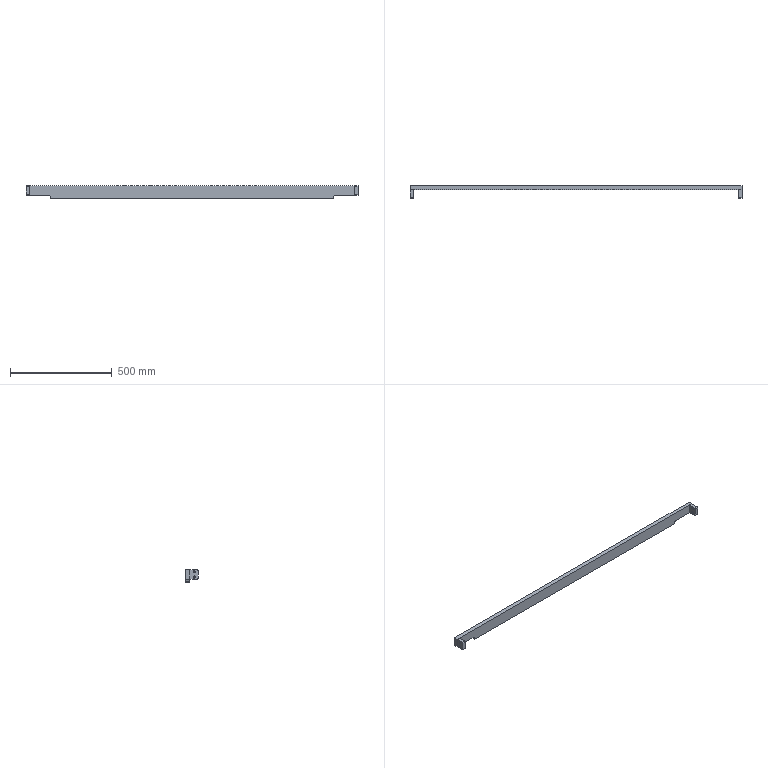Part | SolidWorks | features BaseBody 3 | 3 solids | 36 faces | box 1632 x 60 x 60 mm | volume 1939285 mm3 | plane 22 | cylinder 14 | commonest cylinder face diameters 10.2 x8 10 x4 20 x2
STEP:
#1=CARTESIAN_POINT('',(816.,-10.,30.));
#2=VERTEX_POINT('',#1);
#3=CARTESIAN_POINT('',(816.,-10.,-15.));
#4=VERTEX_POINT('',#3);
#5=CARTESIAN_POINT('',(816.,-10.,-30.));
#6=DIRECTION('',(0.,0.,-1.));
#7=VECTOR('',#6,1000.);
#8=LINE('',#5,#7);
#9=EDGE_CURVE('',#2,#4,#8,.T.);
#10=ORIENTED_EDGE('',*,*,#9,.T.);
#11=CARTESIAN_POINT('',(816.,10.,-15.));
#12=VERTEX_POINT('',#11);
#13=CARTESIAN_POINT('',(816.,-10.,-15.));
#14=DIRECTION('',(0.,1.,0.));
#15=VECTOR('',#14,1000.);
#16=LINE('',#13,#15);
#17=EDGE_CURVE('',#4,#12,#16,.T.);
#18=ORIENTED_EDGE('',*,*,#17,.T.);
#19=CARTESIAN_POINT('',(816.,10.,30.));
#20=VERTEX_POINT('',#19);
#21=CARTESIAN_POINT('',(816.,10.,-30.));
#22=DIRECTION('',(0.,0.,-1.));
#23=VECTOR('',#22,1000.);
#24=LINE('',#21,#23);
#25=EDGE_CURVE('',#20,#12,#24,.T.);
#26=ORIENTED_EDGE('',*,*,#25,.F.);
#27=CARTESIAN_POINT('',(816.,10.,30.));
#28=DIRECTION('',(0.,-1.,0.));
#29=VECTOR('',#28,1000.);
#30=LINE('',#27,#29);
#31=EDGE_CURVE('',#20,#2,#30,.T.);
#32=ORIENTED_EDGE('',*,*,#31,.T.);
#33=EDGE_LOOP('',(#10,#18,#26,#32));
#34=FACE_OUTER_BOUND('',#33,.T.);
#35=CARTESIAN_POINT('',(816.,10.,-30.));
#36=DIRECTION('',(-1.,0.,0.));
#37=DIRECTION('',(0.,0.,1.));
#38=AXIS2_PLACEMENT_3D('',#35,#36,#37);
#39=PLANE('',#38);
#40=ADVANCED_FACE('',(#34),#39,.F.);
#41=CARTESIAN_POINT('',(696.,-10.,-30.));
#42=VERTEX_POINT('',#41);
#43=CARTESIAN_POINT('',(-696.,-10.,-30.));
#44=VERTEX_POINT('',#43);
#45=CARTESIAN_POINT('',(-816.,-10.,-30.));
#46=DIRECTION('',(-1.,0.,0.));
#47=VECTOR('',#46,1000.);
#48=LINE('',#45,#47);
#49=EDGE_CURVE('',#42,#44,#48,.T.);
#50=ORIENTED_EDGE('',*,*,#49,.T.);
#51=CARTESIAN_POINT('',(-696.,10.,-30.));
#52=VERTEX_POINT('',#51);
#53=CARTESIAN_POINT('',(-696.,-10.,-30.));
#54=DIRECTION('',(0.,1.,0.));
#55=VECTOR('',#54,1000.);
#56=LINE('',#53,#55);
#57=EDGE_CURVE('',#44,#52,#56,.T.);
#58=ORIENTED_EDGE('',*,*,#57,.T.);
#59=CARTESIAN_POINT('',(696.,10.,-30.));
#60=VERTEX_POINT('',#59);
#61=CARTESIAN_POINT('',(-816.,10.,-30.));
#62=DIRECTION('',(-1.,0.,0.));
#63=VECTOR('',#62,1000.);
#64=LINE('',#61,#63);
#65=EDGE_CURVE('',#60,#52,#64,.T.);
#66=ORIENTED_EDGE('',*,*,#65,.F.);
#67=CARTESIAN_POINT('',(696.,-10.,-30.));
#68=DIRECTION('',(0.,1.,0.));
#69=VECTOR('',#68,1000.);
#70=LINE('',#67,#69);
#71=EDGE_CURVE('',#42,#60,#70,.T.);
#72=ORIENTED_EDGE('',*,*,#71,.F.);
#73=EDGE_LOOP('',(#50,#58,#66,#72));
#74=FACE_OUTER_BOUND('',#73,.T.);
#75=CARTESIAN_POINT('',(-816.,10.,-30.));
#76=DIRECTION('',(0.,0.,1.));
#77=DIRECTION('',(1.,0.,0.));
#78=AXIS2_PLACEMENT_3D('',#75,#76,#77);
#79=PLANE('',#78);
#80=ADVANCED_FACE('',(#74),#79,.F.);
#81=CARTESIAN_POINT('',(-816.,10.,-15.));
#82=VERTEX_POINT('',#81);
#83=CARTESIAN_POINT('',(-816.,10.,30.));
#84=VERTEX_POINT('',#83);
#85=CARTESIAN_POINT('',(-816.,10.,-30.));
#86=DIRECTION('',(0.,0.,1.));
#87=VECTOR('',#86,1000.);
#88=LINE('',#85,#87);
#89=EDGE_CURVE('',#82,#84,#88,.T.);
#90=ORIENTED_EDGE('',*,*,#89,.F.);
#91=CARTESIAN_POINT('',(-816.,-10.,-15.));
#92=VERTEX_POINT('',#91);
#93=CARTESIAN_POINT('',(-816.,-10.,-15.));
#94=DIRECTION('',(0.,1.,0.));
#95=VECTOR('',#94,1000.);
#96=LINE('',#93,#95);
#97=EDGE_CURVE('',#92,#82,#96,.T.);
#98=ORIENTED_EDGE('',*,*,#97,.F.);
#99=CARTESIAN_POINT('',(-816.,-10.,30.));
#100=VERTEX_POINT('',#99);
#101=CARTESIAN_POINT('',(-816.,-10.,-30.));
#102=DIRECTION('',(0.,0.,1.));
#103=VECTOR('',#102,1000.);
#104=LINE('',#101,#103);
#105=EDGE_CURVE('',#92,#100,#104,.T.);
#106=ORIENTED_EDGE('',*,*,#105,.T.);
#107=CARTESIAN_POINT('',(-816.,10.,30.));
#108=DIRECTION('',(0.,-1.,0.));
#109=VECTOR('',#108,1000.);
#110=LINE('',#107,#109);
#111=EDGE_CURVE('',#84,#100,#110,.T.);
#112=ORIENTED_EDGE('',*,*,#111,.F.);
#113=EDGE_LOOP('',(#90,#98,#106,#112));
#114=FACE_OUTER_BOUND('',#113,.T.);
#115=CARTESIAN_POINT('',(-816.,10.,-30.));
#116=DIRECTION('',(1.,0.,0.));
#117=DIRECTION('',(0.,0.,-1.));
#118=AXIS2_PLACEMENT_3D('',#115,#116,#117);
#119=PLANE('',#118);
#120=ADVANCED_FACE('',(#114),#119,.F.);
#121=CARTESIAN_POINT('',(-816.,-10.,30.));
#122=DIRECTION('',(1.,0.,0.));
#123=VECTOR('',#122,1000.);
#124=LINE('',#121,#123);
#125=EDGE_CURVE('',#100,#2,#124,.T.);
#126=ORIENTED_EDGE('',*,*,#125,.T.);
#127=ORIENTED_EDGE('',*,*,#31,.F.);
#128=CARTESIAN_POINT('',(-816.,10.,30.));
#129=DIRECTION('',(1.,0.,0.));
#130=VECTOR('',#129,1000.);
#131=LINE('',#128,#130);
#132=EDGE_CURVE('',#84,#20,#131,.T.);
#133=ORIENTED_EDGE('',*,*,#132,.F.);
#134=ORIENTED_EDGE('',*,*,#111,.T.);
#135=EDGE_LOOP('',(#126,#127,#133,#134));
#136=FACE_OUTER_BOUND('',#135,.T.);
#137=CARTESIAN_POINT('',(-816.,10.,30.));
#138=DIRECTION('',(0.,0.,-1.));
#139=DIRECTION('',(-1.,0.,0.));
#140=AXIS2_PLACEMENT_3D('',#137,#138,#139);
#141=PLANE('',#140);
#142=ADVANCED_FACE('',(#136),#141,.F.);
#143=CARTESIAN_POINT('',(-696.,10.,-25.));
#144=VERTEX_POINT('',#143);
#145=CARTESIAN_POINT('',(-696.,10.,-30.));
#146=DIRECTION('',(0.,0.,-1.));
#147=VECTOR('',#146,1000.);
#148=LINE('',#145,#147);
#149=EDGE_CURVE('',#144,#52,#148,.T.);
#150=ORIENTED_EDGE('',*,*,#149,.F.);
#151=CARTESIAN_POINT('',(-706.,10.,-15.));
#152=VERTEX_POINT('',#151);
#153=CARTESIAN_POINT('',(-706.,10.,-25.));
#154=DIRECTION('',(0.,1.,0.));
#155=DIRECTION('',(0.,0.,1.));
#156=AXIS2_PLACEMENT_3D('',#153,#154,#155);
#157=CIRCLE('',#156,10.);
#158=EDGE_CURVE('',#152,#144,#157,.T.);
#159=ORIENTED_EDGE('',*,*,#158,.F.);
#160=CARTESIAN_POINT('',(-816.,10.,-15.));
#161=DIRECTION('',(1.,0.,0.));
#162=VECTOR('',#161,1000.);
#163=LINE('',#160,#162);
#164=EDGE_CURVE('',#82,#152,#163,.T.);
#165=ORIENTED_EDGE('',*,*,#164,.F.);
#166=ORIENTED_EDGE('',*,*,#89,.T.);
#167=ORIENTED_EDGE('',*,*,#132,.T.);
#168=ORIENTED_EDGE('',*,*,#25,.T.);
#169=CARTESIAN_POINT('',(706.,10.,-15.));
#170=VERTEX_POINT('',#169);
#171=CARTESIAN_POINT('',(816.,10.,-15.));
#172=DIRECTION('',(1.,0.,0.));
#173=VECTOR('',#172,1000.);
#174=LINE('',#171,#173);
#175=EDGE_CURVE('',#170,#12,#174,.T.);
#176=ORIENTED_EDGE('',*,*,#175,.F.);
#177=CARTESIAN_POINT('',(696.,10.,-25.));
#178=VERTEX_POINT('',#177);
#179=CARTESIAN_POINT('',(706.,10.,-25.));
#180=DIRECTION('',(0.,1.,0.));
#181=DIRECTION('',(0.,0.,-1.));
#182=AXIS2_PLACEMENT_3D('',#179,#180,#181);
#183=CIRCLE('',#182,10.);
#184=EDGE_CURVE('',#178,#170,#183,.T.);
#185=ORIENTED_EDGE('',*,*,#184,.F.);
#186=CARTESIAN_POINT('',(696.,10.,-30.));
#187=DIRECTION('',(0.,0.,1.));
#188=VECTOR('',#187,1000.);
#189=LINE('',#186,#188);
#190=EDGE_CURVE('',#60,#178,#189,.T.);
#191=ORIENTED_EDGE('',*,*,#190,.F.);
#192=ORIENTED_EDGE('',*,*,#65,.T.);
#193=EDGE_LOOP('',(#150,#159,#165,#166,#167,#168,#176,#185,#191,#192));
#194=FACE_OUTER_BOUND('',#193,.T.);
#195=CARTESIAN_POINT('',(0.,10.,0.));
#196=DIRECTION('',(0.,1.,0.));
#197=DIRECTION('',(0.,0.,1.));
#198=AXIS2_PLACEMENT_3D('',#195,#196,#197);
#199=PLANE('',#198);
#200=ADVANCED_FACE('',(#194),#199,.T.);
#201=CARTESIAN_POINT('',(-706.,-10.,-15.));
#202=VERTEX_POINT('',#201);
#203=CARTESIAN_POINT('',(-696.,-10.,-25.));
#204=VERTEX_POINT('',#203);
#205=CARTESIAN_POINT('',(-706.,-10.,-25.));
#206=DIRECTION('',(0.,1.,0.));
#207=DIRECTION('',(0.,0.,1.));
#208=AXIS2_PLACEMENT_3D('',#205,#206,#207);
#209=CIRCLE('',#208,10.);
#210=EDGE_CURVE('',#202,#204,#209,.T.);
#211=ORIENTED_EDGE('',*,*,#210,.T.);
#212=CARTESIAN_POINT('',(-696.,-10.,-30.));
#213=DIRECTION('',(0.,0.,-1.));
#214=VECTOR('',#213,1000.);
#215=LINE('',#212,#214);
#216=EDGE_CURVE('',#204,#44,#215,.T.);
#217=ORIENTED_EDGE('',*,*,#216,.T.);
#218=ORIENTED_EDGE('',*,*,#49,.F.);
#219=CARTESIAN_POINT('',(696.,-10.,-25.));
#220=VERTEX_POINT('',#219);
#221=CARTESIAN_POINT('',(696.,-10.,-30.));
#222=DIRECTION('',(0.,0.,1.));
#223=VECTOR('',#222,1000.);
#224=LINE('',#221,#223);
#225=EDGE_CURVE('',#42,#220,#224,.T.);
#226=ORIENTED_EDGE('',*,*,#225,.T.);
#227=CARTESIAN_POINT('',(706.,-10.,-15.));
#228=VERTEX_POINT('',#227);
#229=CARTESIAN_POINT('',(706.,-10.,-25.));
#230=DIRECTION('',(0.,1.,0.));
#231=DIRECTION('',(0.,0.,-1.));
#232=AXIS2_PLACEMENT_3D('',#229,#230,#231);
#233=CIRCLE('',#232,10.);
#234=EDGE_CURVE('',#220,#228,#233,.T.);
#235=ORIENTED_EDGE('',*,*,#234,.T.);
#236=CARTESIAN_POINT('',(816.,-10.,-15.));
#237=DIRECTION('',(1.,0.,0.));
#238=VECTOR('',#237,1000.);
#239=LINE('',#236,#238);
#240=EDGE_CURVE('',#228,#4,#239,.T.);
#241=ORIENTED_EDGE('',*,*,#240,.T.);
#242=ORIENTED_EDGE('',*,*,#9,.F.);
#243=ORIENTED_EDGE('',*,*,#125,.F.);
#244=ORIENTED_EDGE('',*,*,#105,.F.);
#245=CARTESIAN_POINT('',(-816.,-10.,-15.));
#246=DIRECTION('',(1.,0.,0.));
#247=VECTOR('',#246,1000.);
#248=LINE('',#245,#247);
#249=EDGE_CURVE('',#92,#202,#248,.T.);
#250=ORIENTED_EDGE('',*,*,#249,.T.);
#251=EDGE_LOOP('',(#211,#217,#218,#226,#235,#241,#242,#243,#244,#250));
#252=FACE_OUTER_BOUND('',#251,.T.);
#253=CARTESIAN_POINT('',(0.,-10.,0.));
#254=DIRECTION('',(0.,1.,0.));
#255=DIRECTION('',(0.,0.,1.));
#256=AXIS2_PLACEMENT_3D('',#253,#254,#255);
#257=PLANE('',#256);
#258=ADVANCED_FACE('',(#252),#257,.F.);
#259=ORIENTED_EDGE('',*,*,#175,.T.);
#260=ORIENTED_EDGE('',*,*,#17,.F.);
#261=ORIENTED_EDGE('',*,*,#240,.F.);
#262=CARTESIAN_POINT('',(706.,-10.,-15.));
#263=DIRECTION('',(0.,1.,0.));
#264=VECTOR('',#263,1000.);
#265=LINE('',#262,#264);
#266=EDGE_CURVE('',#228,#170,#265,.T.);
#267=ORIENTED_EDGE('',*,*,#266,.T.);
#268=EDGE_LOOP('',(#259,#260,#261,#267));
#269=FACE_OUTER_BOUND('',#268,.T.);
#270=CARTESIAN_POINT('',(816.,-10.,-15.));
#271=DIRECTION('',(0.,0.,1.));
#272=DIRECTION('',(1.,0.,0.));
#273=AXIS2_PLACEMENT_3D('',#270,#271,#272);
#274=PLANE('',#273);
#275=ADVANCED_FACE('',(#269),#274,.F.);
#276=ORIENTED_EDGE('',*,*,#184,.T.);
#277=ORIENTED_EDGE('',*,*,#266,.F.);
#278=ORIENTED_EDGE('',*,*,#234,.F.);
#279=CARTESIAN_POINT('',(696.,-10.,-25.));
#280=DIRECTION('',(0.,1.,0.));
#281=VECTOR('',#280,1000.);
#282=LINE('',#279,#281);
#283=EDGE_CURVE('',#220,#178,#282,.T.);
#284=ORIENTED_EDGE('',*,*,#283,.T.);
#285=EDGE_LOOP('',(#276,#277,#278,#284));
#286=FACE_OUTER_BOUND('',#285,.T.);
#287=CARTESIAN_POINT('',(706.,-10.,-25.));
#288=DIRECTION('',(0.,1.,0.));
#289=DIRECTION('',(0.,0.,1.));
#290=AXIS2_PLACEMENT_3D('',#287,#288,#289);
#291=CYLINDRICAL_SURFACE('',#290,10.);
#292=ADVANCED_FACE('',(#286),#291,.F.);
#293=ORIENTED_EDGE('',*,*,#190,.T.);
#294=ORIENTED_EDGE('',*,*,#283,.F.);
#295=ORIENTED_EDGE('',*,*,#225,.F.);
#296=ORIENTED_EDGE('',*,*,#71,.T.);
#297=EDGE_LOOP('',(#293,#294,#295,#296));
#298=FACE_OUTER_BOUND('',#297,.T.);
#299=CARTESIAN_POINT('',(696.,-10.,-30.));
#300=DIRECTION('',(-1.,0.,0.));
#301=DIRECTION('',(0.,0.,1.));
#302=AXIS2_PLACEMENT_3D('',#299,#300,#301);
#303=PLANE('',#302);
#304=ADVANCED_FACE('',(#298),#303,.F.);
#305=ORIENTED_EDGE('',*,*,#149,.T.);
#306=ORIENTED_EDGE('',*,*,#57,.F.);
#307=ORIENTED_EDGE('',*,*,#216,.F.);
#308=CARTESIAN_POINT('',(-696.,-10.,-25.));
#309=DIRECTION('',(0.,1.,0.));
#310=VECTOR('',#309,1000.);
#311=LINE('',#308,#310);
#312=EDGE_CURVE('',#204,#144,#311,.T.);
#313=ORIENTED_EDGE('',*,*,#312,.T.);
#314=EDGE_LOOP('',(#305,#306,#307,#313));
#315=FACE_OUTER_BOUND('',#314,.T.);
#316=CARTESIAN_POINT('',(-696.,-10.,-30.));
#317=DIRECTION('',(1.,0.,0.));
#318=DIRECTION('',(0.,0.,-1.));
#319=AXIS2_PLACEMENT_3D('',#316,#317,#318);
#320=PLANE('',#319);
#321=ADVANCED_FACE('',(#315),#320,.F.);
#322=ORIENTED_EDGE('',*,*,#158,.T.);
#323=ORIENTED_EDGE('',*,*,#312,.F.);
#324=ORIENTED_EDGE('',*,*,#210,.F.);
#325=CARTESIAN_POINT('',(-706.,-10.,-15.));
#326=DIRECTION('',(0.,1.,0.));
#327=VECTOR('',#326,1000.);
#328=LINE('',#325,#327);
#329=EDGE_CURVE('',#202,#152,#328,.T.);
#330=ORIENTED_EDGE('',*,*,#329,.T.);
#331=EDGE_LOOP('',(#322,#323,#324,#330));
#332=FACE_OUTER_BOUND('',#331,.T.);
#333=CARTESIAN_POINT('',(-706.,-10.,-25.));
#334=DIRECTION('',(0.,1.,0.));
#335=DIRECTION('',(0.,0.,1.));
#336=AXIS2_PLACEMENT_3D('',#333,#334,#335);
#337=CYLINDRICAL_SURFACE('',#336,10.);
#338=ADVANCED_FACE('',(#332),#337,.F.);
#339=ORIENTED_EDGE('',*,*,#164,.T.);
#340=ORIENTED_EDGE('',*,*,#329,.F.);
#341=ORIENTED_EDGE('',*,*,#249,.F.);
#342=ORIENTED_EDGE('',*,*,#97,.T.);
#343=EDGE_LOOP('',(#339,#340,#341,#342));
#344=FACE_OUTER_BOUND('',#343,.T.);
#345=CARTESIAN_POINT('',(-816.,-10.,-15.));
#346=DIRECTION('',(0.,0.,1.));
#347=DIRECTION('',(1.,0.,0.));
#348=AXIS2_PLACEMENT_3D('',#345,#346,#347);
#349=PLANE('',#348);
#350=ADVANCED_FACE('',(#344),#349,.F.);
#351=CLOSED_SHELL('',(#40,#80,#120,#142,#200,#258,#275,#292,#304,#321,#338,#350));
#352=MANIFOLD_SOLID_BREP('',#351);
#353=CARTESIAN_POINT('',(-800.,-30.,14.9));
#354=VERTEX_POINT('',#353);
#355=CARTESIAN_POINT('',(-800.,-30.,25.1));
#356=VERTEX_POINT('',#355);
#357=CARTESIAN_POINT('',(-800.,-30.,20.));
#358=DIRECTION('',(-1.,0.,0.));
#359=DIRECTION('',(0.,0.,1.));
#360=AXIS2_PLACEMENT_3D('',#357,#358,#359);
#361=CIRCLE('',#360,5.1);
#362=EDGE_CURVE('',#354,#356,#361,.T.);
#363=ORIENTED_EDGE('',*,*,#362,.F.);
#364=CARTESIAN_POINT('',(-816.,-30.,14.9));
#365=VERTEX_POINT('',#364);
#366=CARTESIAN_POINT('',(-816.,-30.,14.9));
#367=DIRECTION('',(-1.,0.,0.));
#368=VECTOR('',#367,1000.);
#369=LINE('',#366,#368);
#370=EDGE_CURVE('',#354,#365,#369,.T.);
#371=ORIENTED_EDGE('',*,*,#370,.T.);
#372=CARTESIAN_POINT('',(-816.,-30.,25.1));
#373=VERTEX_POINT('',#372);
#374=CARTESIAN_POINT('',(-816.,-30.,20.));
#375=DIRECTION('',(-1.,0.,0.));
#376=DIRECTION('',(0.,0.,1.));
#377=AXIS2_PLACEMENT_3D('',#374,#375,#376);
#378=CIRCLE('',#377,5.1);
#379=EDGE_CURVE('',#365,#373,#378,.T.);
#380=ORIENTED_EDGE('',*,*,#379,.T.);
#381=CARTESIAN_POINT('',(-816.,-30.,25.1));
#382=DIRECTION('',(-1.,0.,0.));
#383=VECTOR('',#382,1000.);
#384=LINE('',#381,#383);
#385=EDGE_CURVE('',#356,#373,#384,.T.);
#386=ORIENTED_EDGE('',*,*,#385,.F.);
#387=EDGE_LOOP('',(#363,#371,#380,#386));
#388=FACE_OUTER_BOUND('',#387,.T.);
#389=CARTESIAN_POINT('',(-816.,-30.,20.));
#390=DIRECTION('',(-1.,0.,0.));
#391=DIRECTION('',(0.,0.,1.));
#392=AXIS2_PLACEMENT_3D('',#389,#390,#391);
#393=CYLINDRICAL_SURFACE('',#392,5.1);
#394=ADVANCED_FACE('',(#388),#393,.F.);
#395=CARTESIAN_POINT('',(-800.,-30.,-10.1));
#396=VERTEX_POINT('',#395);
#397=CARTESIAN_POINT('',(-800.,-30.,0.1));
#398=VERTEX_POINT('',#397);
#399=CARTESIAN_POINT('',(-800.,-30.,-5.));
#400=DIRECTION('',(-1.,0.,0.));
#401=DIRECTION('',(0.,0.,1.));
#402=AXIS2_PLACEMENT_3D('',#399,#400,#401);
#403=CIRCLE('',#402,5.1);
#404=EDGE_CURVE('',#396,#398,#403,.T.);
#405=ORIENTED_EDGE('',*,*,#404,.F.);
#406=CARTESIAN_POINT('',(-816.,-30.,-10.1));
#407=VERTEX_POINT('',#406);
#408=CARTESIAN_POINT('',(-816.,-30.,-10.1));
#409=DIRECTION('',(-1.,0.,0.));
#410=VECTOR('',#409,1000.);
#411=LINE('',#408,#410);
#412=EDGE_CURVE('',#396,#407,#411,.T.);
#413=ORIENTED_EDGE('',*,*,#412,.T.);
#414=CARTESIAN_POINT('',(-816.,-30.,0.1));
#415=VERTEX_POINT('',#414);
#416=CARTESIAN_POINT('',(-816.,-30.,-5.));
#417=DIRECTION('',(-1.,0.,0.));
#418=DIRECTION('',(0.,0.,1.));
#419=AXIS2_PLACEMENT_3D('',#416,#417,#418);
#420=CIRCLE('',#419,5.1);
#421=EDGE_CURVE('',#407,#415,#420,.T.);
#422=ORIENTED_EDGE('',*,*,#421,.T.);
#423=CARTESIAN_POINT('',(-816.,-30.,0.1));
#424=DIRECTION('',(-1.,0.,0.));
#425=VECTOR('',#424,1000.);
#426=LINE('',#423,#425);
#427=EDGE_CURVE('',#398,#415,#426,.T.);
#428=ORIENTED_EDGE('',*,*,#427,.F.);
#429=EDGE_LOOP('',(#405,#413,#422,#428));
#430=FACE_OUTER_BOUND('',#429,.T.);
#431=CARTESIAN_POINT('',(-816.,-30.,-5.));
#432=DIRECTION('',(-1.,0.,0.));
#433=DIRECTION('',(0.,0.,1.));
#434=AXIS2_PLACEMENT_3D('',#431,#432,#433);
#435=CYLINDRICAL_SURFACE('',#434,5.1);
#436=ADVANCED_FACE('',(#430),#435,.F.);
#437=CARTESIAN_POINT('',(-816.,-10.,-15.));
#438=VERTEX_POINT('',#437);
#439=CARTESIAN_POINT('',(-816.,-45.,-15.));
#440=VERTEX_POINT('',#439);
#441=CARTESIAN_POINT('',(-816.,-10.,-15.));
#442=DIRECTION('',(0.,-1.,0.));
#443=VECTOR('',#442,1000.);
#444=LINE('',#441,#443);
#445=EDGE_CURVE('',#438,#440,#444,.T.);
#446=ORIENTED_EDGE('',*,*,#445,.F.);
#447=CARTESIAN_POINT('',(-800.,-10.,-15.));
#448=VERTEX_POINT('',#447);
#449=CARTESIAN_POINT('',(-800.,-10.,-15.));
#450=DIRECTION('',(-1.,0.,0.));
#451=VECTOR('',#450,1000.);
#452=LINE('',#449,#451);
#453=EDGE_CURVE('',#448,#438,#452,.T.);
#454=ORIENTED_EDGE('',*,*,#453,.F.);
#455=CARTESIAN_POINT('',(-800.,-45.,-15.));
#456=VERTEX_POINT('',#455);
#457=CARTESIAN_POINT('',(-800.,-10.,-15.));
#458=DIRECTION('',(0.,-1.,0.));
#459=VECTOR('',#458,1000.);
#460=LINE('',#457,#459);
#461=EDGE_CURVE('',#448,#456,#460,.T.);
#462=ORIENTED_EDGE('',*,*,#461,.T.);
#463=CARTESIAN_POINT('',(-800.,-45.,-15.));
#464=DIRECTION('',(-1.,0.,0.));
#465=VECTOR('',#464,1000.);
#466=LINE('',#463,#465);
#467=EDGE_CURVE('',#456,#440,#466,.T.);
#468=ORIENTED_EDGE('',*,*,#467,.T.);
#469=EDGE_LOOP('',(#446,#454,#462,#468));
#470=FACE_OUTER_BOUND('',#469,.T.);
#471=CARTESIAN_POINT('',(-800.,-10.,-15.));
#472=DIRECTION('',(0.,0.,-1.));
#473=DIRECTION('',(-1.,0.,0.));
#474=AXIS2_PLACEMENT_3D('',#471,#472,#473);
#475=PLANE('',#474);
#476=ADVANCED_FACE('',(#470),#475,.T.);
#477=CARTESIAN_POINT('',(-816.,-10.,30.));
#478=VERTEX_POINT('',#477);
#479=CARTESIAN_POINT('',(-816.,-10.,-15.));
#480=DIRECTION('',(0.,0.,-1.));
#481=VECTOR('',#480,1000.);
#482=LINE('',#479,#481);
#483=EDGE_CURVE('',#478,#438,#482,.T.);
#484=ORIENTED_EDGE('',*,*,#483,.F.);
#485=CARTESIAN_POINT('',(-800.,-10.,30.));
#486=VERTEX_POINT('',#485);
#487=CARTESIAN_POINT('',(-800.,-10.,30.));
#488=DIRECTION('',(-1.,0.,0.));
#489=VECTOR('',#488,1000.);
#490=LINE('',#487,#489);
#491=EDGE_CURVE('',#486,#478,#490,.T.);
#492=ORIENTED_EDGE('',*,*,#491,.F.);
#493=CARTESIAN_POINT('',(-800.,-10.,-15.));
#494=DIRECTION('',(0.,0.,-1.));
#495=VECTOR('',#494,1000.);
#496=LINE('',#493,#495);
#497=EDGE_CURVE('',#486,#448,#496,.T.);
#498=ORIENTED_EDGE('',*,*,#497,.T.);
#499=ORIENTED_EDGE('',*,*,#453,.T.);
#500=EDGE_LOOP('',(#484,#492,#498,#499));
#501=FACE_OUTER_BOUND('',#500,.T.);
#502=CARTESIAN_POINT('',(-800.,-10.,-15.));
#503=DIRECTION('',(0.,1.,0.));
#504=DIRECTION('',(0.,0.,1.));
#505=AXIS2_PLACEMENT_3D('',#502,#503,#504);
#506=PLANE('',#505);
#507=ADVANCED_FACE('',(#501),#506,.T.);
#508=CARTESIAN_POINT('',(-816.,-45.,30.));
#509=VERTEX_POINT('',#508);
#510=CARTESIAN_POINT('',(-816.,-10.,30.));
#511=DIRECTION('',(0.,1.,0.));
#512=VECTOR('',#511,1000.);
#513=LINE('',#510,#512);
#514=EDGE_CURVE('',#509,#478,#513,.T.);
#515=ORIENTED_EDGE('',*,*,#514,.F.);
#516=CARTESIAN_POINT('',(-800.,-45.,30.));
#517=VERTEX_POINT('',#516);
#518=CARTESIAN_POINT('',(-800.,-45.,30.));
#519=DIRECTION('',(-1.,0.,0.));
#520=VECTOR('',#519,1000.);
#521=LINE('',#518,#520);
#522=EDGE_CURVE('',#517,#509,#521,.T.);
#523=ORIENTED_EDGE('',*,*,#522,.F.);
#524=CARTESIAN_POINT('',(-800.,-10.,30.));
#525=DIRECTION('',(0.,1.,0.));
#526=VECTOR('',#525,1000.);
#527=LINE('',#524,#526);
#528=EDGE_CURVE('',#517,#486,#527,.T.);
#529=ORIENTED_EDGE('',*,*,#528,.T.);
#530=ORIENTED_EDGE('',*,*,#491,.T.);
#531=EDGE_LOOP('',(#515,#523,#529,#530));
#532=FACE_OUTER_BOUND('',#531,.T.);
#533=CARTESIAN_POINT('',(-800.,-10.,30.));
#534=DIRECTION('',(0.,0.,1.));
#535=DIRECTION('',(1.,0.,0.));
#536=AXIS2_PLACEMENT_3D('',#533,#534,#535);
#537=PLANE('',#536);
#538=ADVANCED_FACE('',(#532),#537,.T.);
#539=CARTESIAN_POINT('',(-816.,-50.,25.));
#540=VERTEX_POINT('',#539);
#541=CARTESIAN_POINT('',(-816.,-45.,25.));
#542=DIRECTION('',(-1.,0.,0.));
#543=DIRECTION('',(0.,0.,1.));
#544=AXIS2_PLACEMENT_3D('',#541,#542,#543);
#545=CIRCLE('',#544,5.);
#546=EDGE_CURVE('',#540,#509,#545,.T.);
#547=ORIENTED_EDGE('',*,*,#546,.F.);
#548=CARTESIAN_POINT('',(-800.,-50.,25.));
#549=VERTEX_POINT('',#548);
#550=CARTESIAN_POINT('',(-800.,-50.,25.));
#551=DIRECTION('',(-1.,0.,0.));
#552=VECTOR('',#551,1000.);
#553=LINE('',#550,#552);
#554=EDGE_CURVE('',#549,#540,#553,.T.);
#555=ORIENTED_EDGE('',*,*,#554,.F.);
#556=CARTESIAN_POINT('',(-800.,-45.,25.));
#557=DIRECTION('',(-1.,0.,0.));
#558=DIRECTION('',(0.,0.,1.));
#559=AXIS2_PLACEMENT_3D('',#556,#557,#558);
#560=CIRCLE('',#559,5.);
#561=EDGE_CURVE('',#549,#517,#560,.T.);
#562=ORIENTED_EDGE('',*,*,#561,.T.);
#563=ORIENTED_EDGE('',*,*,#522,.T.);
#564=EDGE_LOOP('',(#547,#555,#562,#563));
#565=FACE_OUTER_BOUND('',#564,.T.);
#566=CARTESIAN_POINT('',(-800.,-45.,25.));
#567=DIRECTION('',(-1.,0.,0.));
#568=DIRECTION('',(0.,0.,1.));
#569=AXIS2_PLACEMENT_3D('',#566,#567,#568);
#570=CYLINDRICAL_SURFACE('',#569,5.);
#571=ADVANCED_FACE('',(#565),#570,.T.);
#572=CARTESIAN_POINT('',(-816.,-50.,-10.));
#573=VERTEX_POINT('',#572);
#574=CARTESIAN_POINT('',(-816.,-50.,-10.));
#575=DIRECTION('',(0.,0.,1.));
#576=VECTOR('',#575,1000.);
#577=LINE('',#574,#576);
#578=EDGE_CURVE('',#573,#540,#577,.T.);
#579=ORIENTED_EDGE('',*,*,#578,.F.);
#580=CARTESIAN_POINT('',(-800.,-50.,-10.));
#581=VERTEX_POINT('',#580);
#582=CARTESIAN_POINT('',(-800.,-50.,-10.));
#583=DIRECTION('',(-1.,0.,0.));
#584=VECTOR('',#583,1000.);
#585=LINE('',#582,#584);
#586=EDGE_CURVE('',#581,#573,#585,.T.);
#587=ORIENTED_EDGE('',*,*,#586,.F.);
#588=CARTESIAN_POINT('',(-800.,-50.,-10.));
#589=DIRECTION('',(0.,0.,1.));
#590=VECTOR('',#589,1000.);
#591=LINE('',#588,#590);
#592=EDGE_CURVE('',#581,#549,#591,.T.);
#593=ORIENTED_EDGE('',*,*,#592,.T.);
#594=ORIENTED_EDGE('',*,*,#554,.T.);
#595=EDGE_LOOP('',(#579,#587,#593,#594));
#596=FACE_OUTER_BOUND('',#595,.T.);
#597=CARTESIAN_POINT('',(-800.,-50.,-10.));
#598=DIRECTION('',(0.,-1.,0.));
#599=DIRECTION('',(0.,0.,-1.));
#600=AXIS2_PLACEMENT_3D('',#597,#598,#599);
#601=PLANE('',#600);
#602=ADVANCED_FACE('',(#596),#601,.T.);
#603=CARTESIAN_POINT('',(-816.,-45.,-10.));
#604=DIRECTION('',(-1.,0.,0.));
#605=DIRECTION('',(0.,0.,1.));
#606=AXIS2_PLACEMENT_3D('',#603,#604,#605);
#607=CIRCLE('',#606,5.);
#608=EDGE_CURVE('',#440,#573,#607,.T.);
#609=ORIENTED_EDGE('',*,*,#608,.F.);
#610=ORIENTED_EDGE('',*,*,#467,.F.);
#611=CARTESIAN_POINT('',(-800.,-45.,-10.));
#612=DIRECTION('',(-1.,0.,0.));
#613=DIRECTION('',(0.,0.,1.));
#614=AXIS2_PLACEMENT_3D('',#611,#612,#613);
#615=CIRCLE('',#614,5.);
#616=EDGE_CURVE('',#456,#581,#615,.T.);
#617=ORIENTED_EDGE('',*,*,#616,.T.);
#618=ORIENTED_EDGE('',*,*,#586,.T.);
#619=EDGE_LOOP('',(#609,#610,#617,#618));
#620=FACE_OUTER_BOUND('',#619,.T.);
#621=CARTESIAN_POINT('',(-800.,-45.,-10.));
#622=DIRECTION('',(-1.,0.,0.));
#623=DIRECTION('',(0.,0.,1.));
#624=AXIS2_PLACEMENT_3D('',#621,#622,#623);
#625=CYLINDRICAL_SURFACE('',#624,5.);
#626=ADVANCED_FACE('',(#620),#625,.T.);
#627=CARTESIAN_POINT('',(-800.,-30.,20.));
#628=DIRECTION('',(-1.,0.,0.));
#629=DIRECTION('',(0.,0.,1.));
#630=AXIS2_PLACEMENT_3D('',#627,#628,#629);
#631=CIRCLE('',#630,5.1);
#632=EDGE_CURVE('',#356,#354,#631,.T.);
#633=ORIENTED_EDGE('',*,*,#632,.T.);
#634=ORIENTED_EDGE('',*,*,#362,.T.);
#635=EDGE_LOOP('',(#633,#634));
#636=FACE_BOUND('',#635,.T.);
#637=CARTESIAN_POINT('',(-800.,-30.,-5.));
#638=DIRECTION('',(-1.,0.,0.));
#639=DIRECTION('',(0.,0.,1.));
#640=AXIS2_PLACEMENT_3D('',#637,#638,#639);
#641=CIRCLE('',#640,5.1);
#642=EDGE_CURVE('',#398,#396,#641,.T.);
#643=ORIENTED_EDGE('',*,*,#642,.T.);
#644=ORIENTED_EDGE('',*,*,#404,.T.);
#645=EDGE_LOOP('',(#643,#644));
#646=FACE_BOUND('',#645,.T.);
#647=ORIENTED_EDGE('',*,*,#461,.F.);
#648=ORIENTED_EDGE('',*,*,#497,.F.);
#649=ORIENTED_EDGE('',*,*,#528,.F.);
#650=ORIENTED_EDGE('',*,*,#561,.F.);
#651=ORIENTED_EDGE('',*,*,#592,.F.);
#652=ORIENTED_EDGE('',*,*,#616,.F.);
#653=EDGE_LOOP('',(#647,#648,#649,#650,#651,#652));
#654=FACE_OUTER_BOUND('',#653,.T.);
#655=CARTESIAN_POINT('',(-800.,-45.,-10.));
#656=DIRECTION('',(-1.,0.,0.));
#657=DIRECTION('',(0.,0.,1.));
#658=AXIS2_PLACEMENT_3D('',#655,#656,#657);
#659=PLANE('',#658);
#660=ADVANCED_FACE('',(#636,#646,#654),#659,.F.);
#661=CARTESIAN_POINT('',(-816.,-30.,20.));
#662=DIRECTION('',(-1.,0.,0.));
#663=DIRECTION('',(0.,0.,1.));
#664=AXIS2_PLACEMENT_3D('',#661,#662,#663);
#665=CIRCLE('',#664,5.1);
#666=EDGE_CURVE('',#373,#365,#665,.T.);
#667=ORIENTED_EDGE('',*,*,#666,.F.);
#668=ORIENTED_EDGE('',*,*,#379,.F.);
#669=EDGE_LOOP('',(#667,#668));
#670=FACE_BOUND('',#669,.T.);
#671=CARTESIAN_POINT('',(-816.,-30.,-5.));
#672=DIRECTION('',(-1.,0.,0.));
#673=DIRECTION('',(0.,0.,1.));
#674=AXIS2_PLACEMENT_3D('',#671,#672,#673);
#675=CIRCLE('',#674,5.1);
#676=EDGE_CURVE('',#415,#407,#675,.T.);
#677=ORIENTED_EDGE('',*,*,#676,.F.);
#678=ORIENTED_EDGE('',*,*,#421,.F.);
#679=EDGE_LOOP('',(#677,#678));
#680=FACE_BOUND('',#679,.T.);
#681=ORIENTED_EDGE('',*,*,#445,.T.);
#682=ORIENTED_EDGE('',*,*,#608,.T.);
#683=ORIENTED_EDGE('',*,*,#578,.T.);
#684=ORIENTED_EDGE('',*,*,#546,.T.);
#685=ORIENTED_EDGE('',*,*,#514,.T.);
#686=ORIENTED_EDGE('',*,*,#483,.T.);
#687=EDGE_LOOP('',(#681,#682,#683,#684,#685,#686));
#688=FACE_OUTER_BOUND('',#687,.T.);
#689=CARTESIAN_POINT('',(-816.,-45.,-10.));
#690=DIRECTION('',(-1.,0.,0.));
#691=DIRECTION('',(0.,0.,1.));
#692=AXIS2_PLACEMENT_3D('',#689,#690,#691);
#693=PLANE('',#692);
#694=ADVANCED_FACE('',(#670,#680,#688),#693,.T.);
#695=ORIENTED_EDGE('',*,*,#412,.F.);
#696=ORIENTED_EDGE('',*,*,#642,.F.);
#697=ORIENTED_EDGE('',*,*,#427,.T.);
#698=ORIENTED_EDGE('',*,*,#676,.T.);
#699=EDGE_LOOP('',(#695,#696,#697,#698));
#700=FACE_OUTER_BOUND('',#699,.T.);
#701=CARTESIAN_POINT('',(-816.,-30.,-5.));
#702=DIRECTION('',(-1.,0.,0.));
#703=DIRECTION('',(0.,0.,1.));
#704=AXIS2_PLACEMENT_3D('',#701,#702,#703);
#705=CYLINDRICAL_SURFACE('',#704,5.1);
#706=ADVANCED_FACE('',(#700),#705,.F.);
#707=ORIENTED_EDGE('',*,*,#370,.F.);
#708=ORIENTED_EDGE('',*,*,#632,.F.);
#709=ORIENTED_EDGE('',*,*,#385,.T.);
#710=ORIENTED_EDGE('',*,*,#666,.T.);
#711=EDGE_LOOP('',(#707,#708,#709,#710));
#712=FACE_OUTER_BOUND('',#711,.T.);
#713=CARTESIAN_POINT('',(-816.,-30.,20.));
#714=DIRECTION('',(-1.,0.,0.));
#715=DIRECTION('',(0.,0.,1.));
#716=AXIS2_PLACEMENT_3D('',#713,#714,#715);
#717=CYLINDRICAL_SURFACE('',#716,5.1);
#718=ADVANCED_FACE('',(#712),#717,.F.);
#719=CLOSED_SHELL('',(#394,#436,#476,#507,#538,#571,#602,#626,#660,#694,#706,#718));
#720=MANIFOLD_SOLID_BREP('',#719);
#721=CARTESIAN_POINT('',(800.,-30.,25.1));
#722=VERTEX_POINT('',#721);
#723=CARTESIAN_POINT('',(800.,-30.,14.9));
#724=VERTEX_POINT('',#723);
#725=CARTESIAN_POINT('',(800.,-30.,20.));
#726=DIRECTION('',(-1.,0.,0.));
#727=DIRECTION('',(0.,0.,1.));
#728=AXIS2_PLACEMENT_3D('',#725,#726,#727);
#729=CIRCLE('',#728,5.1);
#730=EDGE_CURVE('',#722,#724,#729,.T.);
#731=ORIENTED_EDGE('',*,*,#730,.T.);
#732=CARTESIAN_POINT('',(816.,-30.,14.9));
#733=VERTEX_POINT('',#732);
#734=CARTESIAN_POINT('',(816.,-30.,14.9));
#735=DIRECTION('',(1.,0.,0.));
#736=VECTOR('',#735,1000.);
#737=LINE('',#734,#736);
#738=EDGE_CURVE('',#724,#733,#737,.T.);
#739=ORIENTED_EDGE('',*,*,#738,.T.);
#740=CARTESIAN_POINT('',(816.,-30.,25.1));
#741=VERTEX_POINT('',#740);
#742=CARTESIAN_POINT('',(816.,-30.,20.));
#743=DIRECTION('',(-1.,0.,0.));
#744=DIRECTION('',(0.,0.,1.));
#745=AXIS2_PLACEMENT_3D('',#742,#743,#744);
#746=CIRCLE('',#745,5.1);
#747=EDGE_CURVE('',#741,#733,#746,.T.);
#748=ORIENTED_EDGE('',*,*,#747,.F.);
#749=CARTESIAN_POINT('',(816.,-30.,25.1));
#750=DIRECTION('',(1.,0.,0.));
#751=VECTOR('',#750,1000.);
#752=LINE('',#749,#751);
#753=EDGE_CURVE('',#722,#741,#752,.T.);
#754=ORIENTED_EDGE('',*,*,#753,.F.);
#755=EDGE_LOOP('',(#731,#739,#748,#754));
#756=FACE_OUTER_BOUND('',#755,.T.);
#757=CARTESIAN_POINT('',(816.,-30.,20.));
#758=DIRECTION('',(1.,0.,0.));
#759=DIRECTION('',(0.,0.,1.));
#760=AXIS2_PLACEMENT_3D('',#757,#758,#759);
#761=CYLINDRICAL_SURFACE('',#760,5.1);
#762=ADVANCED_FACE('',(#756),#761,.F.);
#763=CARTESIAN_POINT('',(800.,-30.,0.1));
#764=VERTEX_POINT('',#763);
#765=CARTESIAN_POINT('',(800.,-30.,-10.1));
#766=VERTEX_POINT('',#765);
#767=CARTESIAN_POINT('',(800.,-30.,-5.));
#768=DIRECTION('',(-1.,0.,0.));
#769=DIRECTION('',(0.,0.,1.));
#770=AXIS2_PLACEMENT_3D('',#767,#768,#769);
#771=CIRCLE('',#770,5.1);
#772=EDGE_CURVE('',#764,#766,#771,.T.);
#773=ORIENTED_EDGE('',*,*,#772,.T.);
#774=CARTESIAN_POINT('',(816.,-30.,-10.1));
#775=VERTEX_POINT('',#774);
#776=CARTESIAN_POINT('',(816.,-30.,-10.1));
#777=DIRECTION('',(1.,0.,0.));
#778=VECTOR('',#777,1000.);
#779=LINE('',#776,#778);
#780=EDGE_CURVE('',#766,#775,#779,.T.);
#781=ORIENTED_EDGE('',*,*,#780,.T.);
#782=CARTESIAN_POINT('',(816.,-30.,0.1));
#783=VERTEX_POINT('',#782);
#784=CARTESIAN_POINT('',(816.,-30.,-5.));
#785=DIRECTION('',(-1.,0.,0.));
#786=DIRECTION('',(0.,0.,1.));
#787=AXIS2_PLACEMENT_3D('',#784,#785,#786);
#788=CIRCLE('',#787,5.1);
#789=EDGE_CURVE('',#783,#775,#788,.T.);
#790=ORIENTED_EDGE('',*,*,#789,.F.);
#791=CARTESIAN_POINT('',(816.,-30.,0.1));
#792=DIRECTION('',(1.,0.,0.));
#793=VECTOR('',#792,1000.);
#794=LINE('',#791,#793);
#795=EDGE_CURVE('',#764,#783,#794,.T.);
#796=ORIENTED_EDGE('',*,*,#795,.F.);
#797=EDGE_LOOP('',(#773,#781,#790,#796));
#798=FACE_OUTER_BOUND('',#797,.T.);
#799=CARTESIAN_POINT('',(816.,-30.,-5.));
#800=DIRECTION('',(1.,0.,0.));
#801=DIRECTION('',(0.,0.,1.));
#802=AXIS2_PLACEMENT_3D('',#799,#800,#801);
#803=CYLINDRICAL_SURFACE('',#802,5.1);
#804=ADVANCED_FACE('',(#798),#803,.F.);
#805=CARTESIAN_POINT('',(816.,-10.,-15.));
#806=VERTEX_POINT('',#805);
#807=CARTESIAN_POINT('',(816.,-45.,-15.));
#808=VERTEX_POINT('',#807);
#809=CARTESIAN_POINT('',(816.,-10.,-15.));
#810=DIRECTION('',(0.,-1.,0.));
#811=VECTOR('',#810,1000.);
#812=LINE('',#809,#811);
#813=EDGE_CURVE('',#806,#808,#812,.T.);
#814=ORIENTED_EDGE('',*,*,#813,.T.);
#815=CARTESIAN_POINT('',(800.,-45.,-15.));
#816=VERTEX_POINT('',#815);
#817=CARTESIAN_POINT('',(800.,-45.,-15.));
#818=DIRECTION('',(1.,0.,0.));
#819=VECTOR('',#818,1000.);
#820=LINE('',#817,#819);
#821=EDGE_CURVE('',#816,#808,#820,.T.);
#822=ORIENTED_EDGE('',*,*,#821,.F.);
#823=CARTESIAN_POINT('',(800.,-10.,-15.));
#824=VERTEX_POINT('',#823);
#825=CARTESIAN_POINT('',(800.,-10.,-15.));
#826=DIRECTION('',(0.,-1.,0.));
#827=VECTOR('',#826,1000.);
#828=LINE('',#825,#827);
#829=EDGE_CURVE('',#824,#816,#828,.T.);
#830=ORIENTED_EDGE('',*,*,#829,.F.);
#831=CARTESIAN_POINT('',(800.,-10.,-15.));
#832=DIRECTION('',(1.,0.,0.));
#833=VECTOR('',#832,1000.);
#834=LINE('',#831,#833);
#835=EDGE_CURVE('',#824,#806,#834,.T.);
#836=ORIENTED_EDGE('',*,*,#835,.T.);
#837=EDGE_LOOP('',(#814,#822,#830,#836));
#838=FACE_OUTER_BOUND('',#837,.T.);
#839=CARTESIAN_POINT('',(800.,-10.,-15.));
#840=DIRECTION('',(0.,0.,-1.));
#841=DIRECTION('',(1.,0.,0.));
#842=AXIS2_PLACEMENT_3D('',#839,#840,#841);
#843=PLANE('',#842);
#844=ADVANCED_FACE('',(#838),#843,.T.);
#845=CARTESIAN_POINT('',(816.,-10.,30.));
#846=VERTEX_POINT('',#845);
#847=CARTESIAN_POINT('',(816.,-10.,-15.));
#848=DIRECTION('',(0.,0.,-1.));
#849=VECTOR('',#848,1000.);
#850=LINE('',#847,#849);
#851=EDGE_CURVE('',#846,#806,#850,.T.);
#852=ORIENTED_EDGE('',*,*,#851,.T.);
#853=ORIENTED_EDGE('',*,*,#835,.F.);
#854=CARTESIAN_POINT('',(800.,-10.,30.));
#855=VERTEX_POINT('',#854);
#856=CARTESIAN_POINT('',(800.,-10.,-15.));
#857=DIRECTION('',(0.,0.,-1.));
#858=VECTOR('',#857,1000.);
#859=LINE('',#856,#858);
#860=EDGE_CURVE('',#855,#824,#859,.T.);
#861=ORIENTED_EDGE('',*,*,#860,.F.);
#862=CARTESIAN_POINT('',(800.,-10.,30.));
#863=DIRECTION('',(1.,0.,0.));
#864=VECTOR('',#863,1000.);
#865=LINE('',#862,#864);
#866=EDGE_CURVE('',#855,#846,#865,.T.);
#867=ORIENTED_EDGE('',*,*,#866,.T.);
#868=EDGE_LOOP('',(#852,#853,#861,#867));
#869=FACE_OUTER_BOUND('',#868,.T.);
#870=CARTESIAN_POINT('',(800.,-10.,-15.));
#871=DIRECTION('',(0.,1.,0.));
#872=DIRECTION('',(0.,0.,1.));
#873=AXIS2_PLACEMENT_3D('',#870,#871,#872);
#874=PLANE('',#873);
#875=ADVANCED_FACE('',(#869),#874,.T.);
#876=CARTESIAN_POINT('',(816.,-45.,30.));
#877=VERTEX_POINT('',#876);
#878=CARTESIAN_POINT('',(816.,-10.,30.));
#879=DIRECTION('',(0.,1.,0.));
#880=VECTOR('',#879,1000.);
#881=LINE('',#878,#880);
#882=EDGE_CURVE('',#877,#846,#881,.T.);
#883=ORIENTED_EDGE('',*,*,#882,.T.);
#884=ORIENTED_EDGE('',*,*,#866,.F.);
#885=CARTESIAN_POINT('',(800.,-45.,30.));
#886=VERTEX_POINT('',#885);
#887=CARTESIAN_POINT('',(800.,-10.,30.));
#888=DIRECTION('',(0.,1.,0.));
#889=VECTOR('',#888,1000.);
#890=LINE('',#887,#889);
#891=EDGE_CURVE('',#886,#855,#890,.T.);
#892=ORIENTED_EDGE('',*,*,#891,.F.);
#893=CARTESIAN_POINT('',(800.,-45.,30.));
#894=DIRECTION('',(1.,0.,0.));
#895=VECTOR('',#894,1000.);
#896=LINE('',#893,#895);
#897=EDGE_CURVE('',#886,#877,#896,.T.);
#898=ORIENTED_EDGE('',*,*,#897,.T.);
#899=EDGE_LOOP('',(#883,#884,#892,#898));
#900=FACE_OUTER_BOUND('',#899,.T.);
#901=CARTESIAN_POINT('',(800.,-10.,30.));
#902=DIRECTION('',(0.,0.,1.));
#903=DIRECTION('',(-1.,0.,0.));
#904=AXIS2_PLACEMENT_3D('',#901,#902,#903);
#905=PLANE('',#904);
#906=ADVANCED_FACE('',(#900),#905,.T.);
#907=CARTESIAN_POINT('',(816.,-50.,25.));
#908=VERTEX_POINT('',#907);
#909=CARTESIAN_POINT('',(816.,-45.,25.));
#910=DIRECTION('',(-1.,0.,0.));
#911=DIRECTION('',(0.,0.,1.));
#912=AXIS2_PLACEMENT_3D('',#909,#910,#911);
#913=CIRCLE('',#912,5.);
#914=EDGE_CURVE('',#908,#877,#913,.T.);
#915=ORIENTED_EDGE('',*,*,#914,.T.);
#916=ORIENTED_EDGE('',*,*,#897,.F.);
#917=CARTESIAN_POINT('',(800.,-50.,25.));
#918=VERTEX_POINT('',#917);
#919=CARTESIAN_POINT('',(800.,-45.,25.));
#920=DIRECTION('',(-1.,0.,0.));
#921=DIRECTION('',(0.,0.,1.));
#922=AXIS2_PLACEMENT_3D('',#919,#920,#921);
#923=CIRCLE('',#922,5.);
#924=EDGE_CURVE('',#918,#886,#923,.T.);
#925=ORIENTED_EDGE('',*,*,#924,.F.);
#926=CARTESIAN_POINT('',(800.,-50.,25.));
#927=DIRECTION('',(1.,0.,0.));
#928=VECTOR('',#927,1000.);
#929=LINE('',#926,#928);
#930=EDGE_CURVE('',#918,#908,#929,.T.);
#931=ORIENTED_EDGE('',*,*,#930,.T.);
#932=EDGE_LOOP('',(#915,#916,#925,#931));
#933=FACE_OUTER_BOUND('',#932,.T.);
#934=CARTESIAN_POINT('',(800.,-45.,25.));
#935=DIRECTION('',(1.,0.,0.));
#936=DIRECTION('',(0.,0.,1.));
#937=AXIS2_PLACEMENT_3D('',#934,#935,#936);
#938=CYLINDRICAL_SURFACE('',#937,5.);
#939=ADVANCED_FACE('',(#933),#938,.T.);
#940=CARTESIAN_POINT('',(816.,-50.,-10.));
#941=VERTEX_POINT('',#940);
#942=CARTESIAN_POINT('',(816.,-50.,-10.));
#943=DIRECTION('',(0.,0.,1.));
#944=VECTOR('',#943,1000.);
#945=LINE('',#942,#944);
#946=EDGE_CURVE('',#941,#908,#945,.T.);
#947=ORIENTED_EDGE('',*,*,#946,.T.);
#948=ORIENTED_EDGE('',*,*,#930,.F.);
#949=CARTESIAN_POINT('',(800.,-50.,-10.));
#950=VERTEX_POINT('',#949);
#951=CARTESIAN_POINT('',(800.,-50.,-10.));
#952=DIRECTION('',(0.,0.,1.));
#953=VECTOR('',#952,1000.);
#954=LINE('',#951,#953);
#955=EDGE_CURVE('',#950,#918,#954,.T.);
#956=ORIENTED_EDGE('',*,*,#955,.F.);
#957=CARTESIAN_POINT('',(800.,-50.,-10.));
#958=DIRECTION('',(1.,0.,0.));
#959=VECTOR('',#958,1000.);
#960=LINE('',#957,#959);
#961=EDGE_CURVE('',#950,#941,#960,.T.);
#962=ORIENTED_EDGE('',*,*,#961,.T.);
#963=EDGE_LOOP('',(#947,#948,#956,#962));
#964=FACE_OUTER_BOUND('',#963,.T.);
#965=CARTESIAN_POINT('',(800.,-50.,-10.));
#966=DIRECTION('',(0.,-1.,0.));
#967=DIRECTION('',(0.,0.,-1.));
#968=AXIS2_PLACEMENT_3D('',#965,#966,#967);
#969=PLANE('',#968);
#970=ADVANCED_FACE('',(#964),#969,.T.);
#971=CARTESIAN_POINT('',(816.,-45.,-10.));
#972=DIRECTION('',(-1.,0.,0.));
#973=DIRECTION('',(0.,0.,1.));
#974=AXIS2_PLACEMENT_3D('',#971,#972,#973);
#975=CIRCLE('',#974,5.);
#976=EDGE_CURVE('',#808,#941,#975,.T.);
#977=ORIENTED_EDGE('',*,*,#976,.T.);
#978=ORIENTED_EDGE('',*,*,#961,.F.);
#979=CARTESIAN_POINT('',(800.,-45.,-10.));
#980=DIRECTION('',(-1.,0.,0.));
#981=DIRECTION('',(0.,0.,1.));
#982=AXIS2_PLACEMENT_3D('',#979,#980,#981);
#983=CIRCLE('',#982,5.);
#984=EDGE_CURVE('',#816,#950,#983,.T.);
#985=ORIENTED_EDGE('',*,*,#984,.F.);
#986=ORIENTED_EDGE('',*,*,#821,.T.);
#987=EDGE_LOOP('',(#977,#978,#985,#986));
#988=FACE_OUTER_BOUND('',#987,.T.);
#989=CARTESIAN_POINT('',(800.,-45.,-10.));
#990=DIRECTION('',(1.,0.,0.));
#991=DIRECTION('',(0.,0.,1.));
#992=AXIS2_PLACEMENT_3D('',#989,#990,#991);
#993=CYLINDRICAL_SURFACE('',#992,5.);
#994=ADVANCED_FACE('',(#988),#993,.T.);
#995=ORIENTED_EDGE('',*,*,#730,.F.);
#996=CARTESIAN_POINT('',(800.,-30.,20.));
#997=DIRECTION('',(-1.,0.,0.));
#998=DIRECTION('',(0.,0.,1.));
#999=AXIS2_PLACEMENT_3D('',#996,#997,#998);
#1000=CIRCLE('',#999,5.1);
#1001=EDGE_CURVE('',#724,#722,#1000,.T.);
#1002=ORIENTED_EDGE('',*,*,#1001,.F.);
#1003=EDGE_LOOP('',(#995,#1002));
#1004=FACE_BOUND('',#1003,.T.);
#1005=ORIENTED_EDGE('',*,*,#772,.F.);
#1006=CARTESIAN_POINT('',(800.,-30.,-5.));
#1007=DIRECTION('',(-1.,0.,0.));
#1008=DIRECTION('',(0.,0.,1.));
#1009=AXIS2_PLACEMENT_3D('',#1006,#1007,#1008);
#1010=CIRCLE('',#1009,5.1);
#1011=EDGE_CURVE('',#766,#764,#1010,.T.);
#1012=ORIENTED_EDGE('',*,*,#1011,.F.);
#1013=EDGE_LOOP('',(#1005,#1012));
#1014=FACE_BOUND('',#1013,.T.);
#1015=ORIENTED_EDGE('',*,*,#829,.T.);
#1016=ORIENTED_EDGE('',*,*,#984,.T.);
#1017=ORIENTED_EDGE('',*,*,#955,.T.);
#1018=ORIENTED_EDGE('',*,*,#924,.T.);
#1019=ORIENTED_EDGE('',*,*,#891,.T.);
#1020=ORIENTED_EDGE('',*,*,#860,.T.);
#1021=EDGE_LOOP('',(#1015,#1016,#1017,#1018,#1019,#1020));
#1022=FACE_OUTER_BOUND('',#1021,.T.);
#1023=CARTESIAN_POINT('',(800.,-45.,-10.));
#1024=DIRECTION('',(1.,0.,0.));
#1025=DIRECTION('',(0.,0.,1.));
#1026=AXIS2_PLACEMENT_3D('',#1023,#1024,#1025);
#1027=PLANE('',#1026);
#1028=ADVANCED_FACE('',(#1004,#1014,#1022),#1027,.F.);
#1029=ORIENTED_EDGE('',*,*,#747,.T.);
#1030=CARTESIAN_POINT('',(816.,-30.,20.));
#1031=DIRECTION('',(-1.,0.,0.));
#1032=DIRECTION('',(0.,0.,1.));
#1033=AXIS2_PLACEMENT_3D('',#1030,#1031,#1032);
#1034=CIRCLE('',#1033,5.1);
#1035=EDGE_CURVE('',#733,#741,#1034,.T.);
#1036=ORIENTED_EDGE('',*,*,#1035,.T.);
#1037=EDGE_LOOP('',(#1029,#1036));
#1038=FACE_BOUND('',#1037,.T.);
#1039=ORIENTED_EDGE('',*,*,#789,.T.);
#1040=CARTESIAN_POINT('',(816.,-30.,-5.));
#1041=DIRECTION('',(-1.,0.,0.));
#1042=DIRECTION('',(0.,0.,1.));
#1043=AXIS2_PLACEMENT_3D('',#1040,#1041,#1042);
#1044=CIRCLE('',#1043,5.1);
#1045=EDGE_CURVE('',#775,#783,#1044,.T.);
#1046=ORIENTED_EDGE('',*,*,#1045,.T.);
#1047=EDGE_LOOP('',(#1039,#1046));
#1048=FACE_BOUND('',#1047,.T.);
#1049=ORIENTED_EDGE('',*,*,#813,.F.);
#1050=ORIENTED_EDGE('',*,*,#851,.F.);
#1051=ORIENTED_EDGE('',*,*,#882,.F.);
#1052=ORIENTED_EDGE('',*,*,#914,.F.);
#1053=ORIENTED_EDGE('',*,*,#946,.F.);
#1054=ORIENTED_EDGE('',*,*,#976,.F.);
#1055=EDGE_LOOP('',(#1049,#1050,#1051,#1052,#1053,#1054));
#1056=FACE_OUTER_BOUND('',#1055,.T.);
#1057=CARTESIAN_POINT('',(816.,-45.,-10.));
#1058=DIRECTION('',(1.,0.,0.));
#1059=DIRECTION('',(0.,0.,1.));
#1060=AXIS2_PLACEMENT_3D('',#1057,#1058,#1059);
#1061=PLANE('',#1060);
#1062=ADVANCED_FACE('',(#1038,#1048,#1056),#1061,.T.);
#1063=ORIENTED_EDGE('',*,*,#780,.F.);
#1064=ORIENTED_EDGE('',*,*,#1011,.T.);
#1065=ORIENTED_EDGE('',*,*,#795,.T.);
#1066=ORIENTED_EDGE('',*,*,#1045,.F.);
#1067=EDGE_LOOP('',(#1063,#1064,#1065,#1066));
#1068=FACE_OUTER_BOUND('',#1067,.T.);
#1069=CARTESIAN_POINT('',(816.,-30.,-5.));
#1070=DIRECTION('',(1.,0.,0.));
#1071=DIRECTION('',(0.,0.,1.));
#1072=AXIS2_PLACEMENT_3D('',#1069,#1070,#1071);
#1073=CYLINDRICAL_SURFACE('',#1072,5.1);
#1074=ADVANCED_FACE('',(#1068),#1073,.F.);
#1075=ORIENTED_EDGE('',*,*,#738,.F.);
#1076=ORIENTED_EDGE('',*,*,#1001,.T.);
#1077=ORIENTED_EDGE('',*,*,#753,.T.);
#1078=ORIENTED_EDGE('',*,*,#1035,.F.);
#1079=EDGE_LOOP('',(#1075,#1076,#1077,#1078));
#1080=FACE_OUTER_BOUND('',#1079,.T.);
#1081=CARTESIAN_POINT('',(816.,-30.,20.));
#1082=DIRECTION('',(1.,0.,0.));
#1083=DIRECTION('',(0.,0.,1.));
#1084=AXIS2_PLACEMENT_3D('',#1081,#1082,#1083);
#1085=CYLINDRICAL_SURFACE('',#1084,5.1);
#1086=ADVANCED_FACE('',(#1080),#1085,.F.);
#1087=CLOSED_SHELL('',(#762,#804,#844,#875,#906,#939,#970,#994,#1028,#1062,#1074,#1086));
#1088=MANIFOLD_SOLID_BREP('',#1087);
#1089=CARTESIAN_POINT('',(0.,0.,0.));
#1090=DIRECTION('',(0.,0.,1.));
#1091=DIRECTION('',(1.,0.,0.));
#1092=AXIS2_PLACEMENT_3D('',#1089,#1090,#1091);
#1093=(LENGTH_UNIT()NAMED_UNIT(*)SI_UNIT(.MILLI.,.METRE.));
#1094=UNCERTAINTY_MEASURE_WITH_UNIT(LENGTH_MEASURE(0.00001),#1093,'','');
#1095=(NAMED_UNIT(*)PLANE_ANGLE_UNIT()SI_UNIT($,.RADIAN.));
#1096=(NAMED_UNIT(*)SI_UNIT($,.STERADIAN.)SOLID_ANGLE_UNIT());
#1097=(GEOMETRIC_REPRESENTATION_CONTEXT(3)GLOBAL_UNCERTAINTY_ASSIGNED_CONTEXT((#1094))GLOBAL_UNIT_ASSIGNED_CONTEXT((#1093,#1095,#1096))REPRESENTATION_CONTEXT('',''));
#1098=ADVANCED_BREP_SHAPE_REPRESENTATION('',(#352,#720,#1088,#1092),#1097);